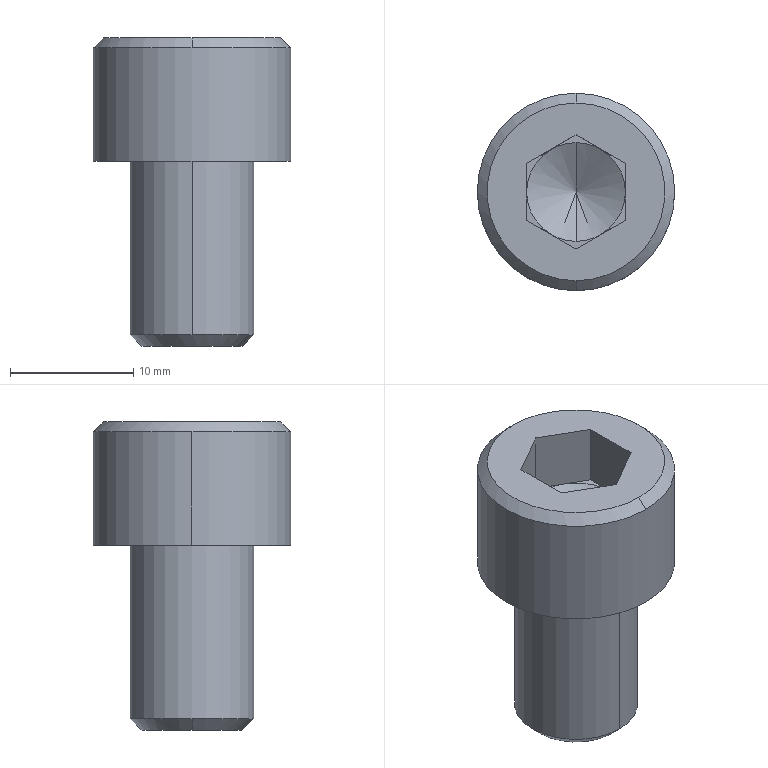Part | STEP file | 1 solid | 25 faces | box 16 x 16 x 25 mm | volume 2845 mm3 | plane 15 | cone 6 | cylinder 4 | commonest cylinder face diameters 10 x2 16 x2